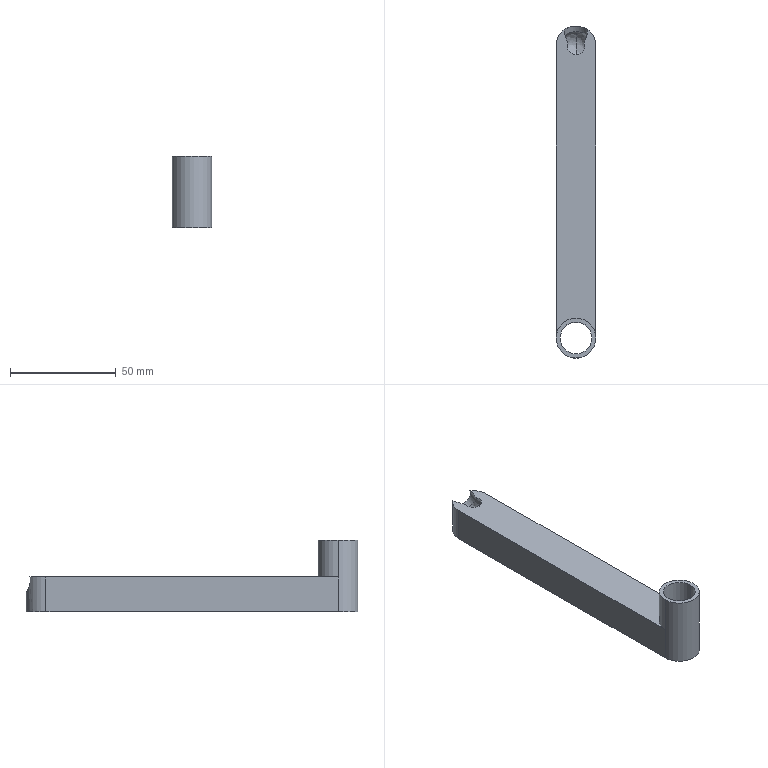Part | SolidWorks | features BaseBody 1 | 1 solid | 13 faces | box 18.898 x 156.922 x 33.625 mm | volume 44298 mm3 | cylinder 6 | plane 5 | spline 2 | commonest cylinder face diameters 18.898 x3 15 x2 11.587 x1
STEP:
#1=CARTESIAN_POINT('',(0.,130.74,10.361));
#2=VERTEX_POINT('',#1);
#3=CARTESIAN_POINT('',(0.,144.777,7.628));
#4=VERTEX_POINT('',#3);
#5=CARTESIAN_POINT('',(0.,138.024,10.361));
#6=DIRECTION('',(1.,0.,0.));
#7=DIRECTION('',(0.,-1.,0.));
#8=AXIS2_PLACEMENT_3D('',#5,#6,#7);
#9=CIRCLE('',#8,7.285);
#10=EDGE_CURVE('',#2,#4,#9,.T.);
#11=ORIENTED_EDGE('',*,*,#10,.F.);
#12=CARTESIAN_POINT('',(0.,133.878,16.35));
#13=VERTEX_POINT('',#12);
#14=CARTESIAN_POINT('',(0.,138.024,10.361));
#15=DIRECTION('',(-1.,0.,0.));
#16=DIRECTION('',(0.,-1.,0.));
#17=AXIS2_PLACEMENT_3D('',#14,#15,#16);
#18=CIRCLE('',#17,7.285);
#19=EDGE_CURVE('',#2,#13,#18,.T.);
#20=ORIENTED_EDGE('',*,*,#19,.T.);
#21=CARTESIAN_POINT('',(3.832,139.608,16.35));
#22=VERTEX_POINT('',#21);
#23=CARTESIAN_POINT('',(3.832,139.608,16.35));
#24=CARTESIAN_POINT('',(3.963,139.291,16.35));
#25=CARTESIAN_POINT('',(4.053,138.965,16.35));
#26=CARTESIAN_POINT('',(4.127,138.463,16.35));
#27=CARTESIAN_POINT('',(4.141,138.292,16.35));
#28=CARTESIAN_POINT('',(4.149,137.952,16.35));
#29=CARTESIAN_POINT('',(4.143,137.782,16.35));
#30=CARTESIAN_POINT('',(4.11,137.446,16.35));
#31=CARTESIAN_POINT('',(4.083,137.28,16.35));
#32=CARTESIAN_POINT('',(4.008,136.949,16.35));
#33=CARTESIAN_POINT('',(3.96,136.783,16.35));
#34=CARTESIAN_POINT('',(3.788,136.304,16.35));
#35=CARTESIAN_POINT('',(3.636,136.003,16.35));
#36=CARTESIAN_POINT('',(3.352,135.578,16.35));
#37=CARTESIAN_POINT('',(3.248,135.441,16.35));
#38=CARTESIAN_POINT('',(3.027,135.185,16.35));
#39=CARTESIAN_POINT('',(2.909,135.064,16.35));
#40=CARTESIAN_POINT('',(2.533,134.724,16.35));
#41=CARTESIAN_POINT('',(2.25,134.525,16.35));
#42=CARTESIAN_POINT('',(1.803,134.287,16.35));
#43=CARTESIAN_POINT('',(1.65,134.216,16.35));
#44=CARTESIAN_POINT('',(1.334,134.095,16.35));
#45=CARTESIAN_POINT('',(1.17,134.043,16.35));
#46=CARTESIAN_POINT('',(0.6745,133.919,16.35));
#47=CARTESIAN_POINT('',(0.3395,133.878,16.35));
#48=CARTESIAN_POINT('',(0.,133.878,16.35));
#49=B_SPLINE_CURVE_WITH_KNOTS('',3,(#23,#24,#25,#26,#27,#28,#29,#30,#31,#32,#33,#34,#35,#36,#37,#38,#39,#40,#41,#42,#43,#44,#45,#46,#47,#48),.UNSPECIFIED.,.F.,.F.,(4,2,2,2,2,2,2,2,2,2,2,2,4),(0.,0.001013,0.001519,0.002025,0.002531,0.003038,0.00405,0.004557,0.005063,0.006075,0.006582,0.007088,0.0081),.UNSPECIFIED.);
#50=EDGE_CURVE('',#22,#13,#49,.T.);
#51=ORIENTED_EDGE('',*,*,#50,.F.);
#52=CARTESIAN_POINT('',(0.,141.823,12.612));
#53=DIRECTION('',(0.,0.8602,0.5099));
#54=DIRECTION('',(0.,-0.5099,0.8602));
#55=AXIS2_PLACEMENT_3D('',#52,#53,#54);
#56=CIRCLE('',#55,5.794);
#57=EDGE_CURVE('',#22,#4,#56,.T.);
#58=ORIENTED_EDGE('',*,*,#57,.T.);
#59=EDGE_LOOP('',(#11,#20,#51,#58));
#60=FACE_OUTER_BOUND('',#59,.T.);
#61=CARTESIAN_POINT('',(0.,130.74,10.361));
#62=CARTESIAN_POINT('',(0.,130.74,10.361));
#63=CARTESIAN_POINT('',(0.,130.74,10.361));
#64=CARTESIAN_POINT('',(0.,130.74,10.361));
#65=CARTESIAN_POINT('',(0.,130.74,-0.1263));
#66=CARTESIAN_POINT('',(20.974,130.74,-0.1263));
#67=CARTESIAN_POINT('',(20.974,130.74,20.848));
#68=CARTESIAN_POINT('',(0.,130.74,20.848));
#69=CARTESIAN_POINT('',(0.,141.05,-2.045));
#70=CARTESIAN_POINT('',(24.81,141.05,-2.045));
#71=CARTESIAN_POINT('',(24.81,141.05,22.766));
#72=CARTESIAN_POINT('',(0.,141.05,22.766));
#73=CARTESIAN_POINT('',(0.,144.822,7.741));
#74=CARTESIAN_POINT('',(5.24,144.822,7.741));
#75=CARTESIAN_POINT('',(5.24,144.822,12.981));
#76=CARTESIAN_POINT('',(0.,144.822,12.981));
#77=(BOUNDED_SURFACE()B_SPLINE_SURFACE(3,3,((#61,#62,#63,#64),(#65,#66,#67,#68),(#69,#70,#71,#72),(#73,#74,#75,#76)),.UNSPECIFIED.,.F.,.F.,.F.)B_SPLINE_SURFACE_WITH_KNOTS((4,4),(4,4),(0.,1.),(0.,1.),.UNSPECIFIED.)GEOMETRIC_REPRESENTATION_ITEM()RATIONAL_B_SPLINE_SURFACE(((1.,0.3333,0.3333,1.),(0.4553,0.1518,0.1518,0.4553),(0.4553,0.1518,0.1518,0.4553),(1.,0.3333,0.3333,1.)))REPRESENTATION_ITEM('')SURFACE());
#78=ADVANCED_FACE('',(#60),#77,.F.);
#79=CARTESIAN_POINT('',(7.5,0.,0.));
#80=VERTEX_POINT('',#79);
#81=CARTESIAN_POINT('',(-7.5,0.,0.));
#82=VERTEX_POINT('',#81);
#83=CARTESIAN_POINT('',(0.,0.,0.));
#84=DIRECTION('',(0.,0.,-1.));
#85=DIRECTION('',(1.,0.,0.));
#86=AXIS2_PLACEMENT_3D('',#83,#84,#85);
#87=CIRCLE('',#86,7.5);
#88=EDGE_CURVE('',#80,#82,#87,.T.);
#89=ORIENTED_EDGE('',*,*,#88,.T.);
#90=CARTESIAN_POINT('',(-7.5,0.,33.625));
#91=VERTEX_POINT('',#90);
#92=CARTESIAN_POINT('',(-7.5,0.,0.));
#93=DIRECTION('',(0.,0.,1.));
#94=VECTOR('',#93,1000.);
#95=LINE('',#92,#94);
#96=EDGE_CURVE('',#82,#91,#95,.T.);
#97=ORIENTED_EDGE('',*,*,#96,.T.);
#98=CARTESIAN_POINT('',(7.5,0.,33.625));
#99=VERTEX_POINT('',#98);
#100=CARTESIAN_POINT('',(0.,0.,33.625));
#101=DIRECTION('',(0.,0.,-1.));
#102=DIRECTION('',(1.,0.,0.));
#103=AXIS2_PLACEMENT_3D('',#100,#101,#102);
#104=CIRCLE('',#103,7.5);
#105=EDGE_CURVE('',#99,#91,#104,.T.);
#106=ORIENTED_EDGE('',*,*,#105,.F.);
#107=CARTESIAN_POINT('',(7.5,0.,0.));
#108=DIRECTION('',(0.,0.,1.));
#109=VECTOR('',#108,1000.);
#110=LINE('',#107,#109);
#111=EDGE_CURVE('',#80,#99,#110,.T.);
#112=ORIENTED_EDGE('',*,*,#111,.F.);
#113=EDGE_LOOP('',(#89,#97,#106,#112));
#114=FACE_OUTER_BOUND('',#113,.T.);
#115=CARTESIAN_POINT('',(0.,0.,0.));
#116=DIRECTION('',(0.,0.,1.));
#117=DIRECTION('',(1.,0.,0.));
#118=AXIS2_PLACEMENT_3D('',#115,#116,#117);
#119=CYLINDRICAL_SURFACE('',#118,7.5);
#120=ADVANCED_FACE('',(#114),#119,.F.);
#121=CARTESIAN_POINT('',(9.449,0.,16.35));
#122=VERTEX_POINT('',#121);
#123=CARTESIAN_POINT('',(-9.449,0.,16.35));
#124=VERTEX_POINT('',#123);
#125=CARTESIAN_POINT('',(0.,0.,16.35));
#126=DIRECTION('',(0.,0.,1.));
#127=DIRECTION('',(1.,0.,0.));
#128=AXIS2_PLACEMENT_3D('',#125,#126,#127);
#129=CIRCLE('',#128,9.449);
#130=EDGE_CURVE('',#122,#124,#129,.T.);
#131=ORIENTED_EDGE('',*,*,#130,.T.);
#132=CARTESIAN_POINT('',(-9.449,0.,33.625));
#133=VERTEX_POINT('',#132);
#134=CARTESIAN_POINT('',(-9.449,0.,0.));
#135=DIRECTION('',(0.,0.,1.));
#136=VECTOR('',#135,1000.);
#137=LINE('',#134,#136);
#138=EDGE_CURVE('',#124,#133,#137,.T.);
#139=ORIENTED_EDGE('',*,*,#138,.T.);
#140=CARTESIAN_POINT('',(9.449,0.,33.625));
#141=VERTEX_POINT('',#140);
#142=CARTESIAN_POINT('',(0.,0.,33.625));
#143=DIRECTION('',(0.,0.,-1.));
#144=DIRECTION('',(1.,0.,0.));
#145=AXIS2_PLACEMENT_3D('',#142,#143,#144);
#146=CIRCLE('',#145,9.449);
#147=EDGE_CURVE('',#133,#141,#146,.T.);
#148=ORIENTED_EDGE('',*,*,#147,.T.);
#149=CARTESIAN_POINT('',(9.449,0.,0.));
#150=DIRECTION('',(0.,0.,1.));
#151=VECTOR('',#150,1000.);
#152=LINE('',#149,#151);
#153=EDGE_CURVE('',#122,#141,#152,.T.);
#154=ORIENTED_EDGE('',*,*,#153,.F.);
#155=EDGE_LOOP('',(#131,#139,#148,#154));
#156=FACE_OUTER_BOUND('',#155,.T.);
#157=CARTESIAN_POINT('',(0.,0.,0.));
#158=DIRECTION('',(0.,0.,1.));
#159=DIRECTION('',(1.,0.,0.));
#160=AXIS2_PLACEMENT_3D('',#157,#158,#159);
#161=CYLINDRICAL_SURFACE('',#160,9.449);
#162=ADVANCED_FACE('',(#156),#161,.T.);
#163=ORIENTED_EDGE('',*,*,#88,.F.);
#164=CARTESIAN_POINT('',(0.,0.,0.));
#165=DIRECTION('',(0.,0.,-1.));
#166=DIRECTION('',(1.,0.,0.));
#167=AXIS2_PLACEMENT_3D('',#164,#165,#166);
#168=CIRCLE('',#167,7.5);
#169=EDGE_CURVE('',#82,#80,#168,.T.);
#170=ORIENTED_EDGE('',*,*,#169,.F.);
#171=EDGE_LOOP('',(#163,#170));
#172=FACE_BOUND('',#171,.T.);
#173=CARTESIAN_POINT('',(9.449,0.,0.));
#174=VERTEX_POINT('',#173);
#175=CARTESIAN_POINT('',(9.449,138.024,0.));
#176=VERTEX_POINT('',#175);
#177=CARTESIAN_POINT('',(9.449,69.012,0.));
#178=DIRECTION('',(0.,1.,0.));
#179=VECTOR('',#178,1000.);
#180=LINE('',#177,#179);
#181=EDGE_CURVE('',#174,#176,#180,.T.);
#182=ORIENTED_EDGE('',*,*,#181,.F.);
#183=CARTESIAN_POINT('',(-9.449,0.,0.));
#184=VERTEX_POINT('',#183);
#185=CARTESIAN_POINT('',(0.,0.,0.));
#186=DIRECTION('',(0.,0.,1.));
#187=DIRECTION('',(1.,0.,0.));
#188=AXIS2_PLACEMENT_3D('',#185,#186,#187);
#189=CIRCLE('',#188,9.449);
#190=EDGE_CURVE('',#184,#174,#189,.T.);
#191=ORIENTED_EDGE('',*,*,#190,.F.);
#192=CARTESIAN_POINT('',(-9.449,138.024,0.));
#193=VERTEX_POINT('',#192);
#194=CARTESIAN_POINT('',(-9.449,69.012,0.));
#195=DIRECTION('',(0.,-1.,0.));
#196=VECTOR('',#195,1000.);
#197=LINE('',#194,#196);
#198=EDGE_CURVE('',#193,#184,#197,.T.);
#199=ORIENTED_EDGE('',*,*,#198,.F.);
#200=CARTESIAN_POINT('',(0.,138.024,0.));
#201=DIRECTION('',(0.,0.,1.));
#202=DIRECTION('',(1.,0.,0.));
#203=AXIS2_PLACEMENT_3D('',#200,#201,#202);
#204=CIRCLE('',#203,9.449);
#205=EDGE_CURVE('',#176,#193,#204,.T.);
#206=ORIENTED_EDGE('',*,*,#205,.F.);
#207=EDGE_LOOP('',(#182,#191,#199,#206));
#208=FACE_OUTER_BOUND('',#207,.T.);
#209=CARTESIAN_POINT('',(0.,69.012,0.));
#210=DIRECTION('',(0.,0.,1.));
#211=DIRECTION('',(1.,0.,0.));
#212=AXIS2_PLACEMENT_3D('',#209,#210,#211);
#213=PLANE('',#212);
#214=ADVANCED_FACE('',(#172,#208),#213,.F.);
#215=ORIENTED_EDGE('',*,*,#96,.F.);
#216=ORIENTED_EDGE('',*,*,#169,.T.);
#217=ORIENTED_EDGE('',*,*,#111,.T.);
#218=CARTESIAN_POINT('',(0.,0.,33.625));
#219=DIRECTION('',(0.,0.,-1.));
#220=DIRECTION('',(1.,0.,0.));
#221=AXIS2_PLACEMENT_3D('',#218,#219,#220);
#222=CIRCLE('',#221,7.5);
#223=EDGE_CURVE('',#91,#99,#222,.T.);
#224=ORIENTED_EDGE('',*,*,#223,.F.);
#225=EDGE_LOOP('',(#215,#216,#217,#224));
#226=FACE_OUTER_BOUND('',#225,.T.);
#227=CARTESIAN_POINT('',(0.,0.,0.));
#228=DIRECTION('',(0.,0.,1.));
#229=DIRECTION('',(1.,0.,0.));
#230=AXIS2_PLACEMENT_3D('',#227,#228,#229);
#231=CYLINDRICAL_SURFACE('',#230,7.5);
#232=ADVANCED_FACE('',(#226),#231,.F.);
#233=CARTESIAN_POINT('',(-9.449,138.024,16.35));
#234=VERTEX_POINT('',#233);
#235=CARTESIAN_POINT('',(-9.449,138.024,0.));
#236=DIRECTION('',(0.,0.,1.));
#237=VECTOR('',#236,1000.);
#238=LINE('',#235,#237);
#239=EDGE_CURVE('',#193,#234,#238,.T.);
#240=ORIENTED_EDGE('',*,*,#239,.T.);
#241=CARTESIAN_POINT('',(-5.648,145.599,16.35));
#242=VERTEX_POINT('',#241);
#243=CARTESIAN_POINT('',(0.,138.024,16.35));
#244=DIRECTION('',(0.,0.,-1.));
#245=DIRECTION('',(1.,0.,0.));
#246=AXIS2_PLACEMENT_3D('',#243,#244,#245);
#247=CIRCLE('',#246,9.449);
#248=EDGE_CURVE('',#234,#242,#247,.T.);
#249=ORIENTED_EDGE('',*,*,#248,.T.);
#250=CARTESIAN_POINT('',(5.648,145.599,16.35));
#251=VERTEX_POINT('',#250);
#252=CARTESIAN_POINT('',(-5.648,145.599,16.35));
#253=CARTESIAN_POINT('',(-5.729,145.539,15.905));
#254=CARTESIAN_POINT('',(-5.778,145.501,15.456));
#255=CARTESIAN_POINT('',(-5.803,145.481,14.553));
#256=CARTESIAN_POINT('',(-5.777,145.502,14.092));
#257=CARTESIAN_POINT('',(-5.668,145.585,13.427));
#258=CARTESIAN_POINT('',(-5.62,145.62,13.209));
#259=CARTESIAN_POINT('',(-5.499,145.709,12.781));
#260=CARTESIAN_POINT('',(-5.425,145.761,12.569));
#261=CARTESIAN_POINT('',(-5.167,145.938,11.962));
#262=CARTESIAN_POINT('',(-4.948,146.08,11.593));
#263=CARTESIAN_POINT('',(-4.546,146.309,11.088));
#264=CARTESIAN_POINT('',(-4.401,146.388,10.93));
#265=CARTESIAN_POINT('',(-4.092,146.543,10.635));
#266=CARTESIAN_POINT('',(-3.929,146.62,10.499));
#267=CARTESIAN_POINT('',(-3.583,146.77,10.245));
#268=CARTESIAN_POINT('',(-3.4,146.843,10.128));
#269=CARTESIAN_POINT('',(-3.021,146.98,9.916));
#270=CARTESIAN_POINT('',(-2.825,147.043,9.821));
#271=CARTESIAN_POINT('',(-2.423,147.16,9.652));
#272=CARTESIAN_POINT('',(-2.215,147.213,9.578));
#273=CARTESIAN_POINT('',(-1.788,147.305,9.45));
#274=CARTESIAN_POINT('',(-1.568,147.345,9.397));
#275=CARTESIAN_POINT('',(-0.907,147.44,9.269));
#276=CARTESIAN_POINT('',(-0.4587,147.473,9.227));
#277=CARTESIAN_POINT('',(0.2252,147.473,9.226));
#278=CARTESIAN_POINT('',(0.4542,147.465,9.237));
#279=CARTESIAN_POINT('',(0.9039,147.433,9.28));
#280=CARTESIAN_POINT('',(1.126,147.409,9.311));
#281=CARTESIAN_POINT('',(1.785,147.314,9.438));
#282=CARTESIAN_POINT('',(2.219,147.219,9.567));
#283=CARTESIAN_POINT('',(3.025,146.986,9.905));
#284=CARTESIAN_POINT('',(3.402,146.848,10.114));
#285=CARTESIAN_POINT('',(4.1,146.546,10.624));
#286=CARTESIAN_POINT('',(4.407,146.388,10.915));
#287=CARTESIAN_POINT('',(4.806,146.161,11.414));
#288=CARTESIAN_POINT('',(4.93,146.086,11.592));
#289=CARTESIAN_POINT('',(5.152,145.946,11.965));
#290=CARTESIAN_POINT('',(5.25,145.881,12.159));
#291=CARTESIAN_POINT('',(5.421,145.764,12.559));
#292=CARTESIAN_POINT('',(5.494,145.712,12.766));
#293=CARTESIAN_POINT('',(5.617,145.623,13.194));
#294=CARTESIAN_POINT('',(5.666,145.586,13.417));
#295=CARTESIAN_POINT('',(5.777,145.502,14.085));
#296=CARTESIAN_POINT('',(5.803,145.482,14.538));
#297=CARTESIAN_POINT('',(5.779,145.5,15.453));
#298=CARTESIAN_POINT('',(5.729,145.539,15.904));
#299=CARTESIAN_POINT('',(5.648,145.599,16.35));
#300=B_SPLINE_CURVE_WITH_KNOTS('',3,(#252,#253,#254,#255,#256,#257,#258,#259,#260,#261,#262,#263,#264,#265,#266,#267,#268,#269,#270,#271,#272,#273,#274,#275,#276,#277,#278,#279,#280,#281,#282,#283,#284,#285,#286,#287,#288,#289,#290,#291,#292,#293,#294,#295,#296,#297,#298,#299),.UNSPECIFIED.,.F.,.F.,(4,2,2,2,2,2,2,2,2,2,2,2,2,2,2,2,2,2,2,2,2,2,2,4),(0.,0.001355,0.00271,0.003388,0.004065,0.00542,0.006098,0.006776,0.007453,0.008131,0.008808,0.009486,0.01084,0.01152,0.0122,0.01355,0.01491,0.01626,0.01694,0.01762,0.01829,0.01897,0.02033,0.02168),.UNSPECIFIED.);
#301=EDGE_CURVE('',#242,#251,#300,.T.);
#302=ORIENTED_EDGE('',*,*,#301,.T.);
#303=CARTESIAN_POINT('',(9.449,138.024,16.35));
#304=VERTEX_POINT('',#303);
#305=CARTESIAN_POINT('',(0.,138.024,16.35));
#306=DIRECTION('',(0.,0.,-1.));
#307=DIRECTION('',(1.,0.,0.));
#308=AXIS2_PLACEMENT_3D('',#305,#306,#307);
#309=CIRCLE('',#308,9.449);
#310=EDGE_CURVE('',#251,#304,#309,.T.);
#311=ORIENTED_EDGE('',*,*,#310,.T.);
#312=CARTESIAN_POINT('',(9.449,138.024,0.));
#313=DIRECTION('',(0.,0.,-1.));
#314=VECTOR('',#313,1000.);
#315=LINE('',#312,#314);
#316=EDGE_CURVE('',#304,#176,#315,.T.);
#317=ORIENTED_EDGE('',*,*,#316,.T.);
#318=ORIENTED_EDGE('',*,*,#205,.T.);
#319=EDGE_LOOP('',(#240,#249,#302,#311,#317,#318));
#320=FACE_OUTER_BOUND('',#319,.T.);
#321=CARTESIAN_POINT('',(0.,138.024,0.));
#322=DIRECTION('',(0.,0.,1.));
#323=DIRECTION('',(1.,0.,0.));
#324=AXIS2_PLACEMENT_3D('',#321,#322,#323);
#325=CYLINDRICAL_SURFACE('',#324,9.449);
#326=ADVANCED_FACE('',(#320),#325,.T.);
#327=CARTESIAN_POINT('',(9.449,0.,16.35));
#328=DIRECTION('',(0.,-1.,0.));
#329=VECTOR('',#328,1000.);
#330=LINE('',#327,#329);
#331=EDGE_CURVE('',#304,#122,#330,.T.);
#332=ORIENTED_EDGE('',*,*,#331,.T.);
#333=CARTESIAN_POINT('',(9.449,0.,0.));
#334=DIRECTION('',(0.,0.,-1.));
#335=VECTOR('',#334,1000.);
#336=LINE('',#333,#335);
#337=EDGE_CURVE('',#122,#174,#336,.T.);
#338=ORIENTED_EDGE('',*,*,#337,.T.);
#339=ORIENTED_EDGE('',*,*,#181,.T.);
#340=ORIENTED_EDGE('',*,*,#316,.F.);
#341=EDGE_LOOP('',(#332,#338,#339,#340));
#342=FACE_OUTER_BOUND('',#341,.T.);
#343=CARTESIAN_POINT('',(9.449,0.,0.));
#344=DIRECTION('',(1.,0.,0.));
#345=DIRECTION('',(0.,0.,-1.));
#346=AXIS2_PLACEMENT_3D('',#343,#344,#345);
#347=PLANE('',#346);
#348=ADVANCED_FACE('',(#342),#347,.T.);
#349=ORIENTED_EDGE('',*,*,#138,.F.);
#350=CARTESIAN_POINT('',(-9.449,0.,0.));
#351=DIRECTION('',(0.,0.,-1.));
#352=VECTOR('',#351,1000.);
#353=LINE('',#350,#352);
#354=EDGE_CURVE('',#124,#184,#353,.T.);
#355=ORIENTED_EDGE('',*,*,#354,.T.);
#356=ORIENTED_EDGE('',*,*,#190,.T.);
#357=ORIENTED_EDGE('',*,*,#337,.F.);
#358=ORIENTED_EDGE('',*,*,#153,.T.);
#359=CARTESIAN_POINT('',(0.,0.,33.625));
#360=DIRECTION('',(0.,0.,-1.));
#361=DIRECTION('',(1.,0.,0.));
#362=AXIS2_PLACEMENT_3D('',#359,#360,#361);
#363=CIRCLE('',#362,9.449);
#364=EDGE_CURVE('',#141,#133,#363,.T.);
#365=ORIENTED_EDGE('',*,*,#364,.T.);
#366=EDGE_LOOP('',(#349,#355,#356,#357,#358,#365));
#367=FACE_OUTER_BOUND('',#366,.T.);
#368=CARTESIAN_POINT('',(0.,0.,0.));
#369=DIRECTION('',(0.,0.,1.));
#370=DIRECTION('',(1.,0.,0.));
#371=AXIS2_PLACEMENT_3D('',#368,#369,#370);
#372=CYLINDRICAL_SURFACE('',#371,9.449);
#373=ADVANCED_FACE('',(#367),#372,.T.);
#374=CARTESIAN_POINT('',(-9.449,138.024,16.35));
#375=DIRECTION('',(0.,1.,0.));
#376=VECTOR('',#375,1000.);
#377=LINE('',#374,#376);
#378=EDGE_CURVE('',#124,#234,#377,.T.);
#379=ORIENTED_EDGE('',*,*,#378,.T.);
#380=ORIENTED_EDGE('',*,*,#239,.F.);
#381=ORIENTED_EDGE('',*,*,#198,.T.);
#382=ORIENTED_EDGE('',*,*,#354,.F.);
#383=EDGE_LOOP('',(#379,#380,#381,#382));
#384=FACE_OUTER_BOUND('',#383,.T.);
#385=CARTESIAN_POINT('',(-9.449,138.024,0.));
#386=DIRECTION('',(-1.,0.,0.));
#387=DIRECTION('',(0.,-1.,0.));
#388=AXIS2_PLACEMENT_3D('',#385,#386,#387);
#389=PLANE('',#388);
#390=ADVANCED_FACE('',(#384),#389,.T.);
#391=ORIENTED_EDGE('',*,*,#105,.T.);
#392=ORIENTED_EDGE('',*,*,#223,.T.);
#393=EDGE_LOOP('',(#391,#392));
#394=FACE_BOUND('',#393,.T.);
#395=ORIENTED_EDGE('',*,*,#364,.F.);
#396=ORIENTED_EDGE('',*,*,#147,.F.);
#397=EDGE_LOOP('',(#395,#396));
#398=FACE_OUTER_BOUND('',#397,.T.);
#399=CARTESIAN_POINT('',(0.,0.,33.625));
#400=DIRECTION('',(0.,0.,-1.));
#401=DIRECTION('',(-1.,0.,0.));
#402=AXIS2_PLACEMENT_3D('',#399,#400,#401);
#403=PLANE('',#402);
#404=ADVANCED_FACE('',(#394,#398),#403,.F.);
#405=ORIENTED_EDGE('',*,*,#331,.F.);
#406=ORIENTED_EDGE('',*,*,#310,.F.);
#407=CARTESIAN_POINT('',(5.648,145.599,16.35));
#408=CARTESIAN_POINT('',(5.376,143.259,16.35));
#409=CARTESIAN_POINT('',(4.75,141.195,16.35));
#410=CARTESIAN_POINT('',(3.832,139.608,16.35));
#411=(BOUNDED_CURVE()B_SPLINE_CURVE(3,(#407,#408,#409,#410),.UNSPECIFIED.,.F.,.T.)B_SPLINE_CURVE_WITH_KNOTS((4,4),(1.795,2.419),.UNSPECIFIED.)CURVE()GEOMETRIC_REPRESENTATION_ITEM()RATIONAL_B_SPLINE_CURVE((1.,0.9679,0.9679,1.))REPRESENTATION_ITEM(''));
#412=EDGE_CURVE('',#251,#22,#411,.T.);
#413=ORIENTED_EDGE('',*,*,#412,.T.);
#414=ORIENTED_EDGE('',*,*,#50,.T.);
#415=CARTESIAN_POINT('',(-3.832,139.608,16.35));
#416=VERTEX_POINT('',#415);
#417=CARTESIAN_POINT('',(0.,133.878,16.35));
#418=CARTESIAN_POINT('',(-0.1696,133.878,16.35));
#419=CARTESIAN_POINT('',(-0.3412,133.888,16.35));
#420=CARTESIAN_POINT('',(-0.6777,133.93,16.35));
#421=CARTESIAN_POINT('',(-0.8436,133.961,16.35));
#422=CARTESIAN_POINT('',(-1.171,134.043,16.35));
#423=CARTESIAN_POINT('',(-1.332,134.094,16.35));
#424=CARTESIAN_POINT('',(-1.65,134.216,16.35));
#425=CARTESIAN_POINT('',(-1.805,134.288,16.35));
#426=CARTESIAN_POINT('',(-2.253,134.527,16.35));
#427=CARTESIAN_POINT('',(-2.529,134.721,16.35));
#428=CARTESIAN_POINT('',(-3.036,135.18,16.35));
#429=CARTESIAN_POINT('',(-3.257,135.436,16.35));
#430=CARTESIAN_POINT('',(-3.633,135.997,16.35));
#431=CARTESIAN_POINT('',(-3.789,136.306,16.35));
#432=CARTESIAN_POINT('',(-3.96,136.782,16.35));
#433=CARTESIAN_POINT('',(-4.007,136.944,16.35));
#434=CARTESIAN_POINT('',(-4.082,137.274,16.35));
#435=CARTESIAN_POINT('',(-4.109,137.444,16.35));
#436=CARTESIAN_POINT('',(-4.16,137.95,16.35));
#437=CARTESIAN_POINT('',(-4.152,138.288,16.35));
#438=CARTESIAN_POINT('',(-4.054,138.961,16.35));
#439=CARTESIAN_POINT('',(-3.963,139.291,16.35));
#440=CARTESIAN_POINT('',(-3.832,139.608,16.35));
#441=B_SPLINE_CURVE_WITH_KNOTS('',3,(#417,#418,#419,#420,#421,#422,#423,#424,#425,#426,#427,#428,#429,#430,#431,#432,#433,#434,#435,#436,#437,#438,#439,#440),.UNSPECIFIED.,.F.,.F.,(4,2,2,2,2,2,2,2,2,2,2,4),(0.0081,0.008606,0.009112,0.009618,0.01012,0.01114,0.01215,0.01316,0.01366,0.01417,0.01518,0.01619),.UNSPECIFIED.);
#442=EDGE_CURVE('',#13,#416,#441,.T.);
#443=ORIENTED_EDGE('',*,*,#442,.T.);
#444=CARTESIAN_POINT('',(-3.832,139.608,16.35));
#445=CARTESIAN_POINT('',(-4.75,141.195,16.35));
#446=CARTESIAN_POINT('',(-5.376,143.259,16.35));
#447=CARTESIAN_POINT('',(-5.648,145.599,16.35));
#448=(BOUNDED_CURVE()B_SPLINE_CURVE(3,(#444,#445,#446,#447),.UNSPECIFIED.,.F.,.F.)B_SPLINE_CURVE_WITH_KNOTS((4,4),(3.864,4.488),.UNSPECIFIED.)CURVE()GEOMETRIC_REPRESENTATION_ITEM()RATIONAL_B_SPLINE_CURVE((1.,0.9679,0.9679,1.))REPRESENTATION_ITEM(''));
#449=EDGE_CURVE('',#416,#242,#448,.T.);
#450=ORIENTED_EDGE('',*,*,#449,.T.);
#451=ORIENTED_EDGE('',*,*,#248,.F.);
#452=ORIENTED_EDGE('',*,*,#378,.F.);
#453=ORIENTED_EDGE('',*,*,#130,.F.);
#454=EDGE_LOOP('',(#405,#406,#413,#414,#443,#450,#451,#452,#453));
#455=FACE_OUTER_BOUND('',#454,.T.);
#456=CARTESIAN_POINT('',(0.,69.012,16.35));
#457=DIRECTION('',(0.,0.,1.));
#458=DIRECTION('',(1.,0.,0.));
#459=AXIS2_PLACEMENT_3D('',#456,#457,#458);
#460=PLANE('',#459);
#461=ADVANCED_FACE('',(#455),#460,.T.);
#462=ORIENTED_EDGE('',*,*,#301,.F.);
#463=ORIENTED_EDGE('',*,*,#449,.F.);
#464=CARTESIAN_POINT('',(0.,141.823,12.612));
#465=DIRECTION('',(0.,0.8602,0.5099));
#466=DIRECTION('',(0.,-0.5099,0.8602));
#467=AXIS2_PLACEMENT_3D('',#464,#465,#466);
#468=CIRCLE('',#467,5.794);
#469=EDGE_CURVE('',#4,#416,#468,.T.);
#470=ORIENTED_EDGE('',*,*,#469,.F.);
#471=ORIENTED_EDGE('',*,*,#57,.F.);
#472=ORIENTED_EDGE('',*,*,#412,.F.);
#473=EDGE_LOOP('',(#462,#463,#470,#471,#472));
#474=FACE_OUTER_BOUND('',#473,.T.);
#475=CARTESIAN_POINT('',(0.,150.843,17.959));
#476=DIRECTION('',(0.,0.8602,0.5099));
#477=DIRECTION('',(0.,-0.5099,0.8602));
#478=AXIS2_PLACEMENT_3D('',#475,#476,#477);
#479=CYLINDRICAL_SURFACE('',#478,5.794);
#480=ADVANCED_FACE('',(#474),#479,.F.);
#481=ORIENTED_EDGE('',*,*,#19,.F.);
#482=ORIENTED_EDGE('',*,*,#10,.T.);
#483=ORIENTED_EDGE('',*,*,#469,.T.);
#484=ORIENTED_EDGE('',*,*,#442,.F.);
#485=EDGE_LOOP('',(#481,#482,#483,#484));
#486=FACE_OUTER_BOUND('',#485,.T.);
#487=CARTESIAN_POINT('',(0.,130.74,10.361));
#488=CARTESIAN_POINT('',(0.,130.74,10.361));
#489=CARTESIAN_POINT('',(0.,130.74,10.361));
#490=CARTESIAN_POINT('',(0.,130.74,10.361));
#491=CARTESIAN_POINT('',(0.,130.74,20.848));
#492=CARTESIAN_POINT('',(-20.974,130.74,20.848));
#493=CARTESIAN_POINT('',(-20.974,130.74,-0.1263));
#494=CARTESIAN_POINT('',(0.,130.74,-0.1263));
#495=CARTESIAN_POINT('',(0.,141.05,22.766));
#496=CARTESIAN_POINT('',(-24.81,141.05,22.766));
#497=CARTESIAN_POINT('',(-24.81,141.05,-2.045));
#498=CARTESIAN_POINT('',(0.,141.05,-2.045));
#499=CARTESIAN_POINT('',(0.,144.822,12.981));
#500=CARTESIAN_POINT('',(-5.24,144.822,12.981));
#501=CARTESIAN_POINT('',(-5.24,144.822,7.741));
#502=CARTESIAN_POINT('',(0.,144.822,7.741));
#503=(BOUNDED_SURFACE()B_SPLINE_SURFACE(3,3,((#487,#488,#489,#490),(#491,#492,#493,#494),(#495,#496,#497,#498),(#499,#500,#501,#502)),.UNSPECIFIED.,.F.,.F.,.F.)B_SPLINE_SURFACE_WITH_KNOTS((4,4),(4,4),(0.,1.),(0.,1.),.UNSPECIFIED.)GEOMETRIC_REPRESENTATION_ITEM()RATIONAL_B_SPLINE_SURFACE(((1.,0.3333,0.3333,1.),(0.4553,0.1518,0.1518,0.4553),(0.4553,0.1518,0.1518,0.4553),(1.,0.3333,0.3333,1.)))REPRESENTATION_ITEM('')SURFACE());
#504=ADVANCED_FACE('',(#486),#503,.F.);
#505=CLOSED_SHELL('',(#78,#120,#162,#214,#232,#326,#348,#373,#390,#404,#461,#480,#504));
#506=MANIFOLD_SOLID_BREP('',#505);
#507=CARTESIAN_POINT('',(0.,0.,0.));
#508=DIRECTION('',(0.,0.,1.));
#509=DIRECTION('',(1.,0.,0.));
#510=AXIS2_PLACEMENT_3D('',#507,#508,#509);
#511=(LENGTH_UNIT()NAMED_UNIT(*)SI_UNIT(.MILLI.,.METRE.));
#512=UNCERTAINTY_MEASURE_WITH_UNIT(LENGTH_MEASURE(0.00001),#511,'','');
#513=(NAMED_UNIT(*)PLANE_ANGLE_UNIT()SI_UNIT($,.RADIAN.));
#514=(NAMED_UNIT(*)SI_UNIT($,.STERADIAN.)SOLID_ANGLE_UNIT());
#515=(GEOMETRIC_REPRESENTATION_CONTEXT(3)GLOBAL_UNCERTAINTY_ASSIGNED_CONTEXT((#512))GLOBAL_UNIT_ASSIGNED_CONTEXT((#511,#513,#514))REPRESENTATION_CONTEXT('',''));
#516=ADVANCED_BREP_SHAPE_REPRESENTATION('',(#506,#510),#515);